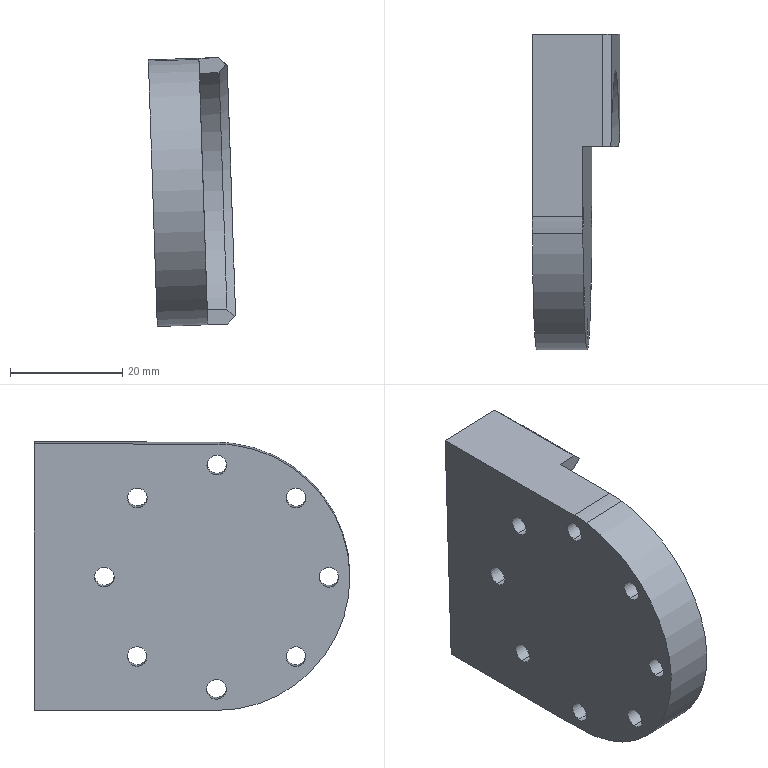Part | STEP file | 2026.6.15-Main Assembly图.sldasm-Part-84 | 1 solid | 42 faces | box 15.538 x 56.282 x 47.929 mm | volume 23654 mm3 | cylinder 27 | plane 14 | cone 1 | commonest cylinder face diameters 3.5 x16 4 x8 47.5 x2 49 x1
STEP:
#1=CARTESIAN_POINT('',(-1524.077,1364.541,3721.229));
#2=VERTEX_POINT('',#1);
#3=CARTESIAN_POINT('',(-1524.077,1364.536,3725.229));
#4=VERTEX_POINT('',#3);
#5=CARTESIAN_POINT('',(-1524.077,1364.538,3723.229));
#6=DIRECTION('',(0.0003632,1.,0.001194));
#7=DIRECTION('',(-0.9994,0.0004028,-0.03334));
#8=AXIS2_PLACEMENT_3D('',#5,#6,#7);
#9=CIRCLE('',#8,2.);
#10=EDGE_CURVE('',#2,#4,#9,.T.);
#11=ORIENTED_EDGE('',*,*,#10,.F.);
#12=CARTESIAN_POINT('',(-1524.075,1372.041,3721.238));
#13=VERTEX_POINT('',#12);
#14=CARTESIAN_POINT('',(-1524.077,1364.541,3721.229));
#15=DIRECTION('',(0.0003632,1.,0.001194));
#16=VECTOR('',#15,1000.);
#17=LINE('',#14,#16);
#18=EDGE_CURVE('',#2,#13,#17,.T.);
#19=ORIENTED_EDGE('',*,*,#18,.T.);
#20=CARTESIAN_POINT('',(-1524.074,1372.036,3725.238));
#21=VERTEX_POINT('',#20);
#22=CARTESIAN_POINT('',(-1524.074,1372.038,3723.238));
#23=DIRECTION('',(-0.0003632,-1.,-0.001194));
#24=DIRECTION('',(-0.9994,0.0004028,-0.03334));
#25=AXIS2_PLACEMENT_3D('',#22,#23,#24);
#26=CIRCLE('',#25,2.);
#27=EDGE_CURVE('',#21,#13,#26,.T.);
#28=ORIENTED_EDGE('',*,*,#27,.F.);
#29=CARTESIAN_POINT('',(-1524.077,1364.536,3725.229));
#30=DIRECTION('',(0.0003632,1.,0.001194));
#31=VECTOR('',#30,1000.);
#32=LINE('',#29,#31);
#33=EDGE_CURVE('',#4,#21,#32,.T.);
#34=ORIENTED_EDGE('',*,*,#33,.F.);
#35=EDGE_LOOP('',(#11,#19,#28,#34));
#36=FACE_OUTER_BOUND('',#35,.T.);
#37=CARTESIAN_POINT('',(-1524.077,1364.538,3723.229));
#38=DIRECTION('',(0.0003632,1.,0.001194));
#39=DIRECTION('',(0.0001943,-0.001194,1.));
#40=AXIS2_PLACEMENT_3D('',#37,#38,#39);
#41=CYLINDRICAL_SURFACE('',#40,2.);
#42=ADVANCED_FACE('',(#36),#41,.F.);
#43=CARTESIAN_POINT('',(-1523.66,1364.551,3712.736));
#44=VERTEX_POINT('',#43);
#45=CARTESIAN_POINT('',(-1523.661,1364.555,3708.736));
#46=VERTEX_POINT('',#45);
#47=CARTESIAN_POINT('',(-1523.66,1364.553,3710.736));
#48=DIRECTION('',(-0.0003632,-1.,-0.001194));
#49=DIRECTION('',(-0.9994,0.0004028,-0.03334));
#50=AXIS2_PLACEMENT_3D('',#47,#48,#49);
#51=CIRCLE('',#50,2.);
#52=EDGE_CURVE('',#44,#46,#51,.T.);
#53=ORIENTED_EDGE('',*,*,#52,.T.);
#54=CARTESIAN_POINT('',(-1523.658,1372.055,3708.745));
#55=VERTEX_POINT('',#54);
#56=CARTESIAN_POINT('',(-1523.661,1364.555,3708.736));
#57=DIRECTION('',(0.0003632,1.,0.001194));
#58=VECTOR('',#57,1000.);
#59=LINE('',#56,#58);
#60=EDGE_CURVE('',#46,#55,#59,.T.);
#61=ORIENTED_EDGE('',*,*,#60,.T.);
#62=CARTESIAN_POINT('',(-1523.657,1372.051,3712.745));
#63=VERTEX_POINT('',#62);
#64=CARTESIAN_POINT('',(-1523.658,1372.053,3710.745));
#65=DIRECTION('',(0.0003632,1.,0.001194));
#66=DIRECTION('',(-0.9994,0.0004028,-0.03334));
#67=AXIS2_PLACEMENT_3D('',#64,#65,#66);
#68=CIRCLE('',#67,2.);
#69=EDGE_CURVE('',#55,#63,#68,.T.);
#70=ORIENTED_EDGE('',*,*,#69,.T.);
#71=CARTESIAN_POINT('',(-1523.66,1364.551,3712.736));
#72=DIRECTION('',(0.0003632,1.,0.001194));
#73=VECTOR('',#72,1000.);
#74=LINE('',#71,#73);
#75=EDGE_CURVE('',#44,#63,#74,.T.);
#76=ORIENTED_EDGE('',*,*,#75,.F.);
#77=EDGE_LOOP('',(#53,#61,#70,#76));
#78=FACE_OUTER_BOUND('',#77,.T.);
#79=CARTESIAN_POINT('',(-1523.66,1364.553,3710.736));
#80=DIRECTION('',(0.0003632,1.,0.001194));
#81=DIRECTION('',(0.0001943,-0.001194,1.));
#82=AXIS2_PLACEMENT_3D('',#79,#80,#81);
#83=CYLINDRICAL_SURFACE('',#82,2.);
#84=ADVANCED_FACE('',(#78),#83,.F.);
#85=CARTESIAN_POINT('',(-1523.243,1364.565,3700.243));
#86=VERTEX_POINT('',#85);
#87=CARTESIAN_POINT('',(-1523.244,1364.57,3696.243));
#88=VERTEX_POINT('',#87);
#89=CARTESIAN_POINT('',(-1523.243,1364.568,3698.243));
#90=DIRECTION('',(-0.0003632,-1.,-0.001194));
#91=DIRECTION('',(-0.9994,0.0004028,-0.03334));
#92=AXIS2_PLACEMENT_3D('',#89,#90,#91);
#93=CIRCLE('',#92,2.);
#94=EDGE_CURVE('',#86,#88,#93,.T.);
#95=ORIENTED_EDGE('',*,*,#94,.T.);
#96=CARTESIAN_POINT('',(-1523.241,1372.07,3696.252));
#97=VERTEX_POINT('',#96);
#98=CARTESIAN_POINT('',(-1523.244,1364.57,3696.243));
#99=DIRECTION('',(0.0003632,1.,0.001194));
#100=VECTOR('',#99,1000.);
#101=LINE('',#98,#100);
#102=EDGE_CURVE('',#88,#97,#101,.T.);
#103=ORIENTED_EDGE('',*,*,#102,.T.);
#104=CARTESIAN_POINT('',(-1523.24,1372.065,3700.252));
#105=VERTEX_POINT('',#104);
#106=CARTESIAN_POINT('',(-1523.241,1372.068,3698.252));
#107=DIRECTION('',(0.0003632,1.,0.001194));
#108=DIRECTION('',(-0.9994,0.0004028,-0.03334));
#109=AXIS2_PLACEMENT_3D('',#106,#107,#108);
#110=CIRCLE('',#109,2.);
#111=EDGE_CURVE('',#97,#105,#110,.T.);
#112=ORIENTED_EDGE('',*,*,#111,.T.);
#113=CARTESIAN_POINT('',(-1523.243,1364.565,3700.243));
#114=DIRECTION('',(0.0003632,1.,0.001194));
#115=VECTOR('',#114,1000.);
#116=LINE('',#113,#115);
#117=EDGE_CURVE('',#86,#105,#116,.T.);
#118=ORIENTED_EDGE('',*,*,#117,.F.);
#119=EDGE_LOOP('',(#95,#103,#112,#118));
#120=FACE_OUTER_BOUND('',#119,.T.);
#121=CARTESIAN_POINT('',(-1523.243,1364.568,3698.243));
#122=DIRECTION('',(0.0003632,1.,0.001194));
#123=DIRECTION('',(0.0001943,-0.001194,1.));
#124=AXIS2_PLACEMENT_3D('',#121,#122,#123);
#125=CYLINDRICAL_SURFACE('',#124,2.);
#126=ADVANCED_FACE('',(#120),#125,.F.);
#127=CARTESIAN_POINT('',(-1522.826,1364.58,3687.75));
#128=VERTEX_POINT('',#127);
#129=CARTESIAN_POINT('',(-1522.827,1364.585,3683.75));
#130=VERTEX_POINT('',#129);
#131=CARTESIAN_POINT('',(-1522.827,1364.583,3685.75));
#132=DIRECTION('',(-0.0003632,-1.,-0.001194));
#133=DIRECTION('',(-0.9994,0.0004028,-0.03334));
#134=AXIS2_PLACEMENT_3D('',#131,#132,#133);
#135=CIRCLE('',#134,2.);
#136=EDGE_CURVE('',#128,#130,#135,.T.);
#137=ORIENTED_EDGE('',*,*,#136,.T.);
#138=CARTESIAN_POINT('',(-1522.824,1372.085,3683.759));
#139=VERTEX_POINT('',#138);
#140=CARTESIAN_POINT('',(-1522.827,1364.585,3683.75));
#141=DIRECTION('',(0.0003632,1.,0.001194));
#142=VECTOR('',#141,1000.);
#143=LINE('',#140,#142);
#144=EDGE_CURVE('',#130,#139,#143,.T.);
#145=ORIENTED_EDGE('',*,*,#144,.T.);
#146=CARTESIAN_POINT('',(-1522.824,1372.08,3687.759));
#147=VERTEX_POINT('',#146);
#148=CARTESIAN_POINT('',(-1522.824,1372.083,3685.759));
#149=DIRECTION('',(0.0003632,1.,0.001194));
#150=DIRECTION('',(-0.9994,0.0004028,-0.03334));
#151=AXIS2_PLACEMENT_3D('',#148,#149,#150);
#152=CIRCLE('',#151,2.);
#153=EDGE_CURVE('',#139,#147,#152,.T.);
#154=ORIENTED_EDGE('',*,*,#153,.T.);
#155=CARTESIAN_POINT('',(-1522.826,1364.58,3687.75));
#156=DIRECTION('',(0.0003632,1.,0.001194));
#157=VECTOR('',#156,1000.);
#158=LINE('',#155,#157);
#159=EDGE_CURVE('',#128,#147,#158,.T.);
#160=ORIENTED_EDGE('',*,*,#159,.F.);
#161=EDGE_LOOP('',(#137,#145,#154,#160));
#162=FACE_OUTER_BOUND('',#161,.T.);
#163=CARTESIAN_POINT('',(-1522.827,1364.583,3685.75));
#164=DIRECTION('',(0.0003632,1.,0.001194));
#165=DIRECTION('',(0.0001943,-0.001194,1.));
#166=AXIS2_PLACEMENT_3D('',#163,#164,#165);
#167=CYLINDRICAL_SURFACE('',#166,2.);
#168=ADVANCED_FACE('',(#162),#167,.F.);
#169=CARTESIAN_POINT('',(-1522.736,1339.811,3682.737));
#170=VERTEX_POINT('',#169);
#171=CARTESIAN_POINT('',(-1522.852,1339.357,3686.205));
#172=VERTEX_POINT('',#171);
#173=CARTESIAN_POINT('',(-1522.794,1339.584,3684.471));
#174=DIRECTION('',(-0.9994,0.0004028,-0.03334));
#175=DIRECTION('',(-0.03311,-0.1296,0.991));
#176=AXIS2_PLACEMENT_3D('',#173,#174,#175);
#177=CIRCLE('',#176,1.75);
#178=EDGE_CURVE('',#170,#172,#177,.T.);
#179=ORIENTED_EDGE('',*,*,#178,.F.);
#180=CARTESIAN_POINT('',(-1531.731,1339.814,3682.436));
#181=VERTEX_POINT('',#180);
#182=CARTESIAN_POINT('',(-1517.739,1339.809,3682.903));
#183=DIRECTION('',(-0.9994,0.0004028,-0.03334));
#184=VECTOR('',#183,1000.);
#185=LINE('',#182,#184);
#186=EDGE_CURVE('',#170,#181,#185,.T.);
#187=ORIENTED_EDGE('',*,*,#186,.T.);
#188=CARTESIAN_POINT('',(-1531.847,1339.361,3685.905));
#189=VERTEX_POINT('',#188);
#190=CARTESIAN_POINT('',(-1531.789,1339.588,3684.171));
#191=DIRECTION('',(0.9994,-0.0004028,0.03334));
#192=DIRECTION('',(-0.03334,-0.001181,0.9994));
#193=AXIS2_PLACEMENT_3D('',#190,#191,#192);
#194=CIRCLE('',#193,1.75);
#195=EDGE_CURVE('',#189,#181,#194,.T.);
#196=ORIENTED_EDGE('',*,*,#195,.F.);
#197=CARTESIAN_POINT('',(-1517.855,1339.355,3686.372));
#198=DIRECTION('',(-0.9994,0.0004028,-0.03334));
#199=VECTOR('',#198,1000.);
#200=LINE('',#197,#199);
#201=EDGE_CURVE('',#172,#189,#200,.T.);
#202=ORIENTED_EDGE('',*,*,#201,.F.);
#203=EDGE_LOOP('',(#179,#187,#196,#202));
#204=FACE_OUTER_BOUND('',#203,.T.);
#205=CARTESIAN_POINT('',(-1517.797,1339.582,3684.637));
#206=DIRECTION('',(-0.9994,0.0004028,-0.03334));
#207=DIRECTION('',(-0.03311,-0.1296,0.991));
#208=AXIS2_PLACEMENT_3D('',#205,#206,#207);
#209=CYLINDRICAL_SURFACE('',#208,1.75);
#210=ADVANCED_FACE('',(#204),#209,.F.);
#211=CARTESIAN_POINT('',(-1524.07,1339.764,3722.714));
#212=VERTEX_POINT('',#211);
#213=CARTESIAN_POINT('',(-1524.186,1339.31,3726.183));
#214=VERTEX_POINT('',#213);
#215=CARTESIAN_POINT('',(-1524.128,1339.537,3724.449));
#216=DIRECTION('',(-0.9994,0.0004028,-0.03334));
#217=DIRECTION('',(-0.03311,-0.1296,0.991));
#218=AXIS2_PLACEMENT_3D('',#215,#216,#217);
#219=CIRCLE('',#218,1.75);
#220=EDGE_CURVE('',#212,#214,#219,.T.);
#221=ORIENTED_EDGE('',*,*,#220,.F.);
#222=CARTESIAN_POINT('',(-1533.065,1339.767,3722.414));
#223=VERTEX_POINT('',#222);
#224=CARTESIAN_POINT('',(-1519.073,1339.762,3722.881));
#225=DIRECTION('',(-0.9994,0.0004028,-0.03334));
#226=VECTOR('',#225,1000.);
#227=LINE('',#224,#226);
#228=EDGE_CURVE('',#212,#223,#227,.T.);
#229=ORIENTED_EDGE('',*,*,#228,.T.);
#230=CARTESIAN_POINT('',(-1533.181,1339.314,3725.883));
#231=VERTEX_POINT('',#230);
#232=CARTESIAN_POINT('',(-1533.123,1339.54,3724.148));
#233=DIRECTION('',(0.9994,-0.0004028,0.03334));
#234=DIRECTION('',(-0.03334,-0.001181,0.9994));
#235=AXIS2_PLACEMENT_3D('',#232,#233,#234);
#236=CIRCLE('',#235,1.75);
#237=EDGE_CURVE('',#231,#223,#236,.T.);
#238=ORIENTED_EDGE('',*,*,#237,.F.);
#239=CARTESIAN_POINT('',(-1519.188,1339.308,3726.349));
#240=DIRECTION('',(-0.9994,0.0004028,-0.03334));
#241=VECTOR('',#240,1000.);
#242=LINE('',#239,#241);
#243=EDGE_CURVE('',#214,#231,#242,.T.);
#244=ORIENTED_EDGE('',*,*,#243,.F.);
#245=EDGE_LOOP('',(#221,#229,#238,#244));
#246=FACE_OUTER_BOUND('',#245,.T.);
#247=CARTESIAN_POINT('',(-1519.131,1339.535,3724.615));
#248=DIRECTION('',(-0.9994,0.0004028,-0.03334));
#249=DIRECTION('',(-0.03311,-0.1296,0.991));
#250=AXIS2_PLACEMENT_3D('',#247,#248,#249);
#251=CYLINDRICAL_SURFACE('',#250,1.75);
#252=ADVANCED_FACE('',(#246),#251,.F.);
#253=CARTESIAN_POINT('',(-1523.88,1325.628,3716.843));
#254=VERTEX_POINT('',#253);
#255=CARTESIAN_POINT('',(-1523.996,1325.175,3720.311));
#256=VERTEX_POINT('',#255);
#257=CARTESIAN_POINT('',(-1523.938,1325.402,3718.577));
#258=DIRECTION('',(-0.9994,0.0004028,-0.03334));
#259=DIRECTION('',(-0.03311,-0.1296,0.991));
#260=AXIS2_PLACEMENT_3D('',#257,#258,#259);
#261=CIRCLE('',#260,1.75);
#262=EDGE_CURVE('',#254,#256,#261,.T.);
#263=ORIENTED_EDGE('',*,*,#262,.F.);
#264=CARTESIAN_POINT('',(-1532.875,1325.632,3716.543));
#265=VERTEX_POINT('',#264);
#266=CARTESIAN_POINT('',(-1518.882,1325.626,3717.009));
#267=DIRECTION('',(-0.9994,0.0004028,-0.03334));
#268=VECTOR('',#267,1000.);
#269=LINE('',#266,#268);
#270=EDGE_CURVE('',#254,#265,#269,.T.);
#271=ORIENTED_EDGE('',*,*,#270,.T.);
#272=CARTESIAN_POINT('',(-1532.991,1325.178,3720.011));
#273=VERTEX_POINT('',#272);
#274=CARTESIAN_POINT('',(-1532.933,1325.405,3718.277));
#275=DIRECTION('',(0.9994,-0.0004028,0.03334));
#276=DIRECTION('',(-0.03334,-0.001181,0.9994));
#277=AXIS2_PLACEMENT_3D('',#274,#275,#276);
#278=CIRCLE('',#277,1.75);
#279=EDGE_CURVE('',#273,#265,#278,.T.);
#280=ORIENTED_EDGE('',*,*,#279,.F.);
#281=CARTESIAN_POINT('',(-1518.998,1325.173,3720.478));
#282=DIRECTION('',(-0.9994,0.0004028,-0.03334));
#283=VECTOR('',#282,1000.);
#284=LINE('',#281,#283);
#285=EDGE_CURVE('',#256,#273,#284,.T.);
#286=ORIENTED_EDGE('',*,*,#285,.F.);
#287=EDGE_LOOP('',(#263,#271,#280,#286));
#288=FACE_OUTER_BOUND('',#287,.T.);
#289=CARTESIAN_POINT('',(-1518.94,1325.4,3718.744));
#290=DIRECTION('',(-0.9994,0.0004028,-0.03334));
#291=DIRECTION('',(-0.03311,-0.1296,0.991));
#292=AXIS2_PLACEMENT_3D('',#289,#290,#291);
#293=CYLINDRICAL_SURFACE('',#292,1.75);
#294=ADVANCED_FACE('',(#288),#293,.F.);
#295=CARTESIAN_POINT('',(-1523.869,1353.913,3716.877));
#296=VERTEX_POINT('',#295);
#297=CARTESIAN_POINT('',(-1523.985,1353.459,3720.345));
#298=VERTEX_POINT('',#297);
#299=CARTESIAN_POINT('',(-1523.927,1353.686,3718.611));
#300=DIRECTION('',(-0.9994,0.0004028,-0.03334));
#301=DIRECTION('',(-0.03311,-0.1296,0.991));
#302=AXIS2_PLACEMENT_3D('',#299,#300,#301);
#303=CIRCLE('',#302,1.75);
#304=EDGE_CURVE('',#296,#298,#303,.T.);
#305=ORIENTED_EDGE('',*,*,#304,.F.);
#306=CARTESIAN_POINT('',(-1532.864,1353.916,3716.576));
#307=VERTEX_POINT('',#306);
#308=CARTESIAN_POINT('',(-1518.872,1353.911,3717.043));
#309=DIRECTION('',(-0.9994,0.0004028,-0.03334));
#310=VECTOR('',#309,1000.);
#311=LINE('',#308,#310);
#312=EDGE_CURVE('',#296,#307,#311,.T.);
#313=ORIENTED_EDGE('',*,*,#312,.T.);
#314=CARTESIAN_POINT('',(-1532.98,1353.463,3720.045));
#315=VERTEX_POINT('',#314);
#316=CARTESIAN_POINT('',(-1532.922,1353.69,3718.311));
#317=DIRECTION('',(0.9994,-0.0004028,0.03334));
#318=DIRECTION('',(-0.03334,-0.001181,0.9994));
#319=AXIS2_PLACEMENT_3D('',#316,#317,#318);
#320=CIRCLE('',#319,1.75);
#321=EDGE_CURVE('',#315,#307,#320,.T.);
#322=ORIENTED_EDGE('',*,*,#321,.F.);
#323=CARTESIAN_POINT('',(-1518.988,1353.457,3720.512));
#324=DIRECTION('',(-0.9994,0.0004028,-0.03334));
#325=VECTOR('',#324,1000.);
#326=LINE('',#323,#325);
#327=EDGE_CURVE('',#298,#315,#326,.T.);
#328=ORIENTED_EDGE('',*,*,#327,.F.);
#329=EDGE_LOOP('',(#305,#313,#322,#328));
#330=FACE_OUTER_BOUND('',#329,.T.);
#331=CARTESIAN_POINT('',(-1518.93,1353.684,3718.777));
#332=DIRECTION('',(-0.9994,0.0004028,-0.03334));
#333=DIRECTION('',(-0.03311,-0.1296,0.991));
#334=AXIS2_PLACEMENT_3D('',#331,#332,#333);
#335=CYLINDRICAL_SURFACE('',#334,1.75);
#336=ADVANCED_FACE('',(#330),#335,.F.);
#337=CARTESIAN_POINT('',(-1523.41,1319.787,3702.702));
#338=VERTEX_POINT('',#337);
#339=CARTESIAN_POINT('',(-1523.526,1319.334,3706.17));
#340=VERTEX_POINT('',#339);
#341=CARTESIAN_POINT('',(-1523.468,1319.56,3704.436));
#342=DIRECTION('',(-0.9994,0.0004028,-0.03334));
#343=DIRECTION('',(-0.03311,-0.1296,0.991));
#344=AXIS2_PLACEMENT_3D('',#341,#342,#343);
#345=CIRCLE('',#344,1.75);
#346=EDGE_CURVE('',#338,#340,#345,.T.);
#347=ORIENTED_EDGE('',*,*,#346,.F.);
#348=CARTESIAN_POINT('',(-1532.405,1319.791,3702.401));
#349=VERTEX_POINT('',#348);
#350=CARTESIAN_POINT('',(-1518.413,1319.785,3702.868));
#351=DIRECTION('',(-0.9994,0.0004028,-0.03334));
#352=VECTOR('',#351,1000.);
#353=LINE('',#350,#352);
#354=EDGE_CURVE('',#338,#349,#353,.T.);
#355=ORIENTED_EDGE('',*,*,#354,.T.);
#356=CARTESIAN_POINT('',(-1532.521,1319.337,3705.87));
#357=VERTEX_POINT('',#356);
#358=CARTESIAN_POINT('',(-1532.463,1319.564,3704.136));
#359=DIRECTION('',(0.9994,-0.0004028,0.03334));
#360=DIRECTION('',(-0.03334,-0.001181,0.9994));
#361=AXIS2_PLACEMENT_3D('',#358,#359,#360);
#362=CIRCLE('',#361,1.75);
#363=EDGE_CURVE('',#357,#349,#362,.T.);
#364=ORIENTED_EDGE('',*,*,#363,.F.);
#365=CARTESIAN_POINT('',(-1518.529,1319.332,3706.337));
#366=DIRECTION('',(-0.9994,0.0004028,-0.03334));
#367=VECTOR('',#366,1000.);
#368=LINE('',#365,#367);
#369=EDGE_CURVE('',#340,#357,#368,.T.);
#370=ORIENTED_EDGE('',*,*,#369,.F.);
#371=EDGE_LOOP('',(#347,#355,#364,#370));
#372=FACE_OUTER_BOUND('',#371,.T.);
#373=CARTESIAN_POINT('',(-1518.471,1319.558,3704.602));
#374=DIRECTION('',(-0.9994,0.0004028,-0.03334));
#375=DIRECTION('',(-0.03311,-0.1296,0.991));
#376=AXIS2_PLACEMENT_3D('',#373,#374,#375);
#377=CYLINDRICAL_SURFACE('',#376,1.75);
#378=ADVANCED_FACE('',(#372),#377,.F.);
#379=CARTESIAN_POINT('',(-1523.396,1359.787,3702.749));
#380=VERTEX_POINT('',#379);
#381=CARTESIAN_POINT('',(-1523.512,1359.334,3706.218));
#382=VERTEX_POINT('',#381);
#383=CARTESIAN_POINT('',(-1523.454,1359.56,3704.484));
#384=DIRECTION('',(-0.9994,0.0004028,-0.03334));
#385=DIRECTION('',(-0.03311,-0.1296,0.991));
#386=AXIS2_PLACEMENT_3D('',#383,#384,#385);
#387=CIRCLE('',#386,1.75);
#388=EDGE_CURVE('',#380,#382,#387,.T.);
#389=ORIENTED_EDGE('',*,*,#388,.F.);
#390=CARTESIAN_POINT('',(-1532.391,1359.791,3702.449));
#391=VERTEX_POINT('',#390);
#392=CARTESIAN_POINT('',(-1518.399,1359.785,3702.916));
#393=DIRECTION('',(-0.9994,0.0004028,-0.03334));
#394=VECTOR('',#393,1000.);
#395=LINE('',#392,#394);
#396=EDGE_CURVE('',#380,#391,#395,.T.);
#397=ORIENTED_EDGE('',*,*,#396,.T.);
#398=CARTESIAN_POINT('',(-1532.507,1359.337,3705.918));
#399=VERTEX_POINT('',#398);
#400=CARTESIAN_POINT('',(-1532.449,1359.564,3704.183));
#401=DIRECTION('',(0.9994,-0.0004028,0.03334));
#402=DIRECTION('',(-0.03334,-0.001181,0.9994));
#403=AXIS2_PLACEMENT_3D('',#400,#401,#402);
#404=CIRCLE('',#403,1.75);
#405=EDGE_CURVE('',#399,#391,#404,.T.);
#406=ORIENTED_EDGE('',*,*,#405,.F.);
#407=CARTESIAN_POINT('',(-1518.514,1359.332,3706.385));
#408=DIRECTION('',(-0.9994,0.0004028,-0.03334));
#409=VECTOR('',#408,1000.);
#410=LINE('',#407,#409);
#411=EDGE_CURVE('',#382,#399,#410,.T.);
#412=ORIENTED_EDGE('',*,*,#411,.F.);
#413=EDGE_LOOP('',(#389,#397,#406,#412));
#414=FACE_OUTER_BOUND('',#413,.T.);
#415=CARTESIAN_POINT('',(-1518.456,1359.558,3704.65));
#416=DIRECTION('',(-0.9994,0.0004028,-0.03334));
#417=DIRECTION('',(-0.03311,-0.1296,0.991));
#418=AXIS2_PLACEMENT_3D('',#415,#416,#417);
#419=CYLINDRICAL_SURFACE('',#418,1.75);
#420=ADVANCED_FACE('',(#414),#419,.F.);
#421=CARTESIAN_POINT('',(-1522.937,1325.662,3688.574));
#422=VERTEX_POINT('',#421);
#423=CARTESIAN_POINT('',(-1523.053,1325.208,3692.043));
#424=VERTEX_POINT('',#423);
#425=CARTESIAN_POINT('',(-1522.995,1325.435,3690.309));
#426=DIRECTION('',(-0.9994,0.0004028,-0.03334));
#427=DIRECTION('',(-0.03311,-0.1296,0.991));
#428=AXIS2_PLACEMENT_3D('',#425,#426,#427);
#429=CIRCLE('',#428,1.75);
#430=EDGE_CURVE('',#422,#424,#429,.T.);
#431=ORIENTED_EDGE('',*,*,#430,.F.);
#432=CARTESIAN_POINT('',(-1531.932,1325.665,3688.274));
#433=VERTEX_POINT('',#432);
#434=CARTESIAN_POINT('',(-1517.939,1325.66,3688.741));
#435=DIRECTION('',(-0.9994,0.0004028,-0.03334));
#436=VECTOR('',#435,1000.);
#437=LINE('',#434,#436);
#438=EDGE_CURVE('',#422,#433,#437,.T.);
#439=ORIENTED_EDGE('',*,*,#438,.T.);
#440=CARTESIAN_POINT('',(-1532.048,1325.212,3691.743));
#441=VERTEX_POINT('',#440);
#442=CARTESIAN_POINT('',(-1531.99,1325.439,3690.008));
#443=DIRECTION('',(0.9994,-0.0004028,0.03334));
#444=DIRECTION('',(-0.03334,-0.001181,0.9994));
#445=AXIS2_PLACEMENT_3D('',#442,#443,#444);
#446=CIRCLE('',#445,1.75);
#447=EDGE_CURVE('',#441,#433,#446,.T.);
#448=ORIENTED_EDGE('',*,*,#447,.F.);
#449=CARTESIAN_POINT('',(-1518.055,1325.206,3692.209));
#450=DIRECTION('',(-0.9994,0.0004028,-0.03334));
#451=VECTOR('',#450,1000.);
#452=LINE('',#449,#451);
#453=EDGE_CURVE('',#424,#441,#452,.T.);
#454=ORIENTED_EDGE('',*,*,#453,.F.);
#455=EDGE_LOOP('',(#431,#439,#448,#454));
#456=FACE_OUTER_BOUND('',#455,.T.);
#457=CARTESIAN_POINT('',(-1517.997,1325.433,3690.475));
#458=DIRECTION('',(-0.9994,0.0004028,-0.03334));
#459=DIRECTION('',(-0.03311,-0.1296,0.991));
#460=AXIS2_PLACEMENT_3D('',#457,#458,#459);
#461=CYLINDRICAL_SURFACE('',#460,1.75);
#462=ADVANCED_FACE('',(#456),#461,.F.);
#463=CARTESIAN_POINT('',(-1522.926,1353.946,3688.608));
#464=VERTEX_POINT('',#463);
#465=CARTESIAN_POINT('',(-1523.042,1353.493,3692.077));
#466=VERTEX_POINT('',#465);
#467=CARTESIAN_POINT('',(-1522.984,1353.719,3690.342));
#468=DIRECTION('',(-0.9994,0.0004028,-0.03334));
#469=DIRECTION('',(-0.03311,-0.1296,0.991));
#470=AXIS2_PLACEMENT_3D('',#467,#468,#469);
#471=CIRCLE('',#470,1.75);
#472=EDGE_CURVE('',#464,#466,#471,.T.);
#473=ORIENTED_EDGE('',*,*,#472,.F.);
#474=CARTESIAN_POINT('',(-1531.921,1353.95,3688.308));
#475=VERTEX_POINT('',#474);
#476=CARTESIAN_POINT('',(-1517.929,1353.944,3688.775));
#477=DIRECTION('',(-0.9994,0.0004028,-0.03334));
#478=VECTOR('',#477,1000.);
#479=LINE('',#476,#478);
#480=EDGE_CURVE('',#464,#475,#479,.T.);
#481=ORIENTED_EDGE('',*,*,#480,.T.);
#482=CARTESIAN_POINT('',(-1532.037,1353.496,3691.776));
#483=VERTEX_POINT('',#482);
#484=CARTESIAN_POINT('',(-1531.979,1353.723,3690.042));
#485=DIRECTION('',(0.9994,-0.0004028,0.03334));
#486=DIRECTION('',(-0.03334,-0.001181,0.9994));
#487=AXIS2_PLACEMENT_3D('',#484,#485,#486);
#488=CIRCLE('',#487,1.75);
#489=EDGE_CURVE('',#483,#475,#488,.T.);
#490=ORIENTED_EDGE('',*,*,#489,.F.);
#491=CARTESIAN_POINT('',(-1518.045,1353.49,3692.243));
#492=DIRECTION('',(-0.9994,0.0004028,-0.03334));
#493=VECTOR('',#492,1000.);
#494=LINE('',#491,#493);
#495=EDGE_CURVE('',#466,#483,#494,.T.);
#496=ORIENTED_EDGE('',*,*,#495,.F.);
#497=EDGE_LOOP('',(#473,#481,#490,#496));
#498=FACE_OUTER_BOUND('',#497,.T.);
#499=CARTESIAN_POINT('',(-1517.987,1353.717,3690.509));
#500=DIRECTION('',(-0.9994,0.0004028,-0.03334));
#501=DIRECTION('',(-0.03311,-0.1296,0.991));
#502=AXIS2_PLACEMENT_3D('',#499,#500,#501);
#503=CYLINDRICAL_SURFACE('',#502,1.75);
#504=ADVANCED_FACE('',(#498),#503,.F.);
#505=CARTESIAN_POINT('',(-1522.669,1339.589,3680.723));
#506=VERTEX_POINT('',#505);
#507=CARTESIAN_POINT('',(-1524.247,1336.483,3727.996));
#508=VERTEX_POINT('',#507);
#509=CARTESIAN_POINT('',(-1523.461,1339.56,3704.46));
#510=DIRECTION('',(-0.9994,0.0004028,-0.03334));
#511=DIRECTION('',(-0.03334,-0.001181,0.9994));
#512=AXIS2_PLACEMENT_3D('',#509,#510,#511);
#513=CIRCLE('',#512,23.75);
#514=EDGE_CURVE('',#506,#508,#513,.T.);
#515=ORIENTED_EDGE('',*,*,#514,.T.);
#516=CARTESIAN_POINT('',(-1533.242,1336.486,3727.696));
#517=VERTEX_POINT('',#516);
#518=CARTESIAN_POINT('',(-1519.25,1336.481,3728.163));
#519=DIRECTION('',(-0.9994,0.0004028,-0.03334));
#520=VECTOR('',#519,1000.);
#521=LINE('',#518,#520);
#522=EDGE_CURVE('',#508,#517,#521,.T.);
#523=ORIENTED_EDGE('',*,*,#522,.T.);
#524=CARTESIAN_POINT('',(-1531.664,1339.592,3680.423));
#525=VERTEX_POINT('',#524);
#526=CARTESIAN_POINT('',(-1532.456,1339.564,3704.16));
#527=DIRECTION('',(-0.9994,0.0004028,-0.03334));
#528=DIRECTION('',(-0.03334,-0.001181,0.9994));
#529=AXIS2_PLACEMENT_3D('',#526,#527,#528);
#530=CIRCLE('',#529,23.75);
#531=EDGE_CURVE('',#525,#517,#530,.T.);
#532=ORIENTED_EDGE('',*,*,#531,.F.);
#533=CARTESIAN_POINT('',(-1517.672,1339.586,3680.89));
#534=DIRECTION('',(-0.9994,0.0004028,-0.03334));
#535=VECTOR('',#534,1000.);
#536=LINE('',#533,#535);
#537=EDGE_CURVE('',#506,#525,#536,.T.);
#538=ORIENTED_EDGE('',*,*,#537,.F.);
#539=EDGE_LOOP('',(#515,#523,#532,#538));
#540=FACE_OUTER_BOUND('',#539,.T.);
#541=CARTESIAN_POINT('',(-1518.464,1339.558,3704.626));
#542=DIRECTION('',(-0.9994,0.0004028,-0.03334));
#543=DIRECTION('',(-0.03311,-0.1296,0.991));
#544=AXIS2_PLACEMENT_3D('',#541,#542,#543);
#545=CYLINDRICAL_SURFACE('',#544,23.75);
#546=ADVANCED_FACE('',(#540),#545,.T.);
#547=CARTESIAN_POINT('',(-1519.159,1372.087,3680.878));
#548=VERTEX_POINT('',#547);
#549=CARTESIAN_POINT('',(-1531.652,1372.092,3680.462));
#550=VERTEX_POINT('',#549);
#551=CARTESIAN_POINT('',(-1517.66,1372.086,3680.928));
#552=DIRECTION('',(-0.9994,0.0004028,-0.03334));
#553=VECTOR('',#552,1000.);
#554=LINE('',#551,#553);
#555=EDGE_CURVE('',#548,#550,#554,.T.);
#556=ORIENTED_EDGE('',*,*,#555,.F.);
#557=CARTESIAN_POINT('',(-1519.167,1352.087,3680.854));
#558=VERTEX_POINT('',#557);
#559=CARTESIAN_POINT('',(-1519.167,1352.087,3680.854));
#560=DIRECTION('',(-0.0003632,-1.,-0.001194));
#561=VECTOR('',#560,1000.);
#562=LINE('',#559,#561);
#563=EDGE_CURVE('',#548,#558,#562,.T.);
#564=ORIENTED_EDGE('',*,*,#563,.T.);
#565=CARTESIAN_POINT('',(-1522.665,1352.088,3680.738));
#566=VERTEX_POINT('',#565);
#567=CARTESIAN_POINT('',(-1517.667,1352.086,3680.904));
#568=DIRECTION('',(-0.9994,0.0004028,-0.03334));
#569=VECTOR('',#568,1000.);
#570=LINE('',#567,#569);
#571=EDGE_CURVE('',#558,#566,#570,.T.);
#572=ORIENTED_EDGE('',*,*,#571,.T.);
#573=CARTESIAN_POINT('',(-1522.665,1352.088,3680.738));
#574=DIRECTION('',(-0.0003632,-1.,-0.001194));
#575=VECTOR('',#574,1000.);
#576=LINE('',#573,#575);
#577=EDGE_CURVE('',#566,#506,#576,.T.);
#578=ORIENTED_EDGE('',*,*,#577,.T.);
#579=ORIENTED_EDGE('',*,*,#537,.T.);
#580=CARTESIAN_POINT('',(-1531.652,1372.092,3680.462));
#581=DIRECTION('',(-0.0003632,-1.,-0.001194));
#582=VECTOR('',#581,1000.);
#583=LINE('',#580,#582);
#584=EDGE_CURVE('',#550,#525,#583,.T.);
#585=ORIENTED_EDGE('',*,*,#584,.F.);
#586=EDGE_LOOP('',(#556,#564,#572,#578,#579,#585));
#587=FACE_OUTER_BOUND('',#586,.T.);
#588=CARTESIAN_POINT('',(-1517.66,1372.086,3680.928));
#589=DIRECTION('',(0.03334,0.001181,-0.9994));
#590=DIRECTION('',(-0.003979,1.,0.001049));
#591=AXIS2_PLACEMENT_3D('',#588,#589,#590);
#592=PLANE('',#591);
#593=ADVANCED_FACE('',(#587),#592,.T.);
#594=CARTESIAN_POINT('',(-1520.75,1352.031,3728.328));
#595=VERTEX_POINT('',#594);
#596=CARTESIAN_POINT('',(-1524.248,1352.032,3728.211));
#597=VERTEX_POINT('',#596);
#598=CARTESIAN_POINT('',(-1519.251,1352.03,3728.378));
#599=DIRECTION('',(-0.9994,0.0004028,-0.03334));
#600=VECTOR('',#599,1000.);
#601=LINE('',#598,#600);
#602=EDGE_CURVE('',#595,#597,#601,.T.);
#603=ORIENTED_EDGE('',*,*,#602,.F.);
#604=CARTESIAN_POINT('',(-1520.743,1372.031,3728.352));
#605=VERTEX_POINT('',#604);
#606=CARTESIAN_POINT('',(-1520.743,1372.031,3728.352));
#607=DIRECTION('',(0.0003632,1.,0.001194));
#608=VECTOR('',#607,1000.);
#609=LINE('',#606,#608);
#610=EDGE_CURVE('',#595,#605,#609,.T.);
#611=ORIENTED_EDGE('',*,*,#610,.T.);
#612=CARTESIAN_POINT('',(-1533.236,1372.036,3727.935));
#613=VERTEX_POINT('',#612);
#614=CARTESIAN_POINT('',(-1519.244,1372.03,3728.402));
#615=DIRECTION('',(-0.9994,0.0004028,-0.03334));
#616=VECTOR('',#615,1000.);
#617=LINE('',#614,#616);
#618=EDGE_CURVE('',#605,#613,#617,.T.);
#619=ORIENTED_EDGE('',*,*,#618,.T.);
#620=CARTESIAN_POINT('',(-1533.248,1339.536,3727.896));
#621=VERTEX_POINT('',#620);
#622=CARTESIAN_POINT('',(-1533.248,1339.536,3727.896));
#623=DIRECTION('',(0.0003632,1.,0.001194));
#624=VECTOR('',#623,1000.);
#625=LINE('',#622,#624);
#626=EDGE_CURVE('',#621,#613,#625,.T.);
#627=ORIENTED_EDGE('',*,*,#626,.F.);
#628=CARTESIAN_POINT('',(-1524.253,1339.532,3728.196));
#629=VERTEX_POINT('',#628);
#630=CARTESIAN_POINT('',(-1519.256,1339.53,3728.363));
#631=DIRECTION('',(-0.9994,0.0004028,-0.03334));
#632=VECTOR('',#631,1000.);
#633=LINE('',#630,#632);
#634=EDGE_CURVE('',#629,#621,#633,.T.);
#635=ORIENTED_EDGE('',*,*,#634,.F.);
#636=CARTESIAN_POINT('',(-1524.253,1339.532,3728.196));
#637=DIRECTION('',(0.0003632,1.,0.001194));
#638=VECTOR('',#637,1000.);
#639=LINE('',#636,#638);
#640=EDGE_CURVE('',#629,#597,#639,.T.);
#641=ORIENTED_EDGE('',*,*,#640,.T.);
#642=EDGE_LOOP('',(#603,#611,#619,#627,#635,#641));
#643=FACE_OUTER_BOUND('',#642,.T.);
#644=CARTESIAN_POINT('',(-1519.256,1339.53,3728.363));
#645=DIRECTION('',(-0.03334,-0.001181,0.9994));
#646=DIRECTION('',(0.003979,-1.,-0.001049));
#647=AXIS2_PLACEMENT_3D('',#644,#645,#646);
#648=PLANE('',#647);
#649=ADVANCED_FACE('',(#643),#648,.T.);
#650=ORIENTED_EDGE('',*,*,#522,.F.);
#651=CARTESIAN_POINT('',(-1523.461,1339.56,3704.46));
#652=DIRECTION('',(-0.9994,0.0004028,-0.03334));
#653=DIRECTION('',(-0.03334,-0.001181,0.9994));
#654=AXIS2_PLACEMENT_3D('',#651,#652,#653);
#655=CIRCLE('',#654,23.75);
#656=EDGE_CURVE('',#508,#629,#655,.T.);
#657=ORIENTED_EDGE('',*,*,#656,.T.);
#658=ORIENTED_EDGE('',*,*,#634,.T.);
#659=CARTESIAN_POINT('',(-1532.456,1339.564,3704.16));
#660=DIRECTION('',(-0.9994,0.0004028,-0.03334));
#661=DIRECTION('',(-0.03334,-0.001181,0.9994));
#662=AXIS2_PLACEMENT_3D('',#659,#660,#661);
#663=CIRCLE('',#662,23.75);
#664=EDGE_CURVE('',#517,#621,#663,.T.);
#665=ORIENTED_EDGE('',*,*,#664,.F.);
#666=EDGE_LOOP('',(#650,#657,#658,#665));
#667=FACE_OUTER_BOUND('',#666,.T.);
#668=CARTESIAN_POINT('',(-1518.464,1339.558,3704.626));
#669=DIRECTION('',(-0.9994,0.0004028,-0.03334));
#670=DIRECTION('',(-0.03311,-0.1296,0.991));
#671=AXIS2_PLACEMENT_3D('',#668,#669,#670);
#672=CYLINDRICAL_SURFACE('',#671,23.75);
#673=ADVANCED_FACE('',(#667),#672,.T.);
#674=ORIENTED_EDGE('',*,*,#27,.T.);
#675=CARTESIAN_POINT('',(-1524.074,1372.038,3723.238));
#676=DIRECTION('',(-0.0003632,-1.,-0.001194));
#677=DIRECTION('',(-0.9994,0.0004028,-0.03334));
#678=AXIS2_PLACEMENT_3D('',#675,#676,#677);
#679=CIRCLE('',#678,2.);
#680=EDGE_CURVE('',#13,#21,#679,.T.);
#681=ORIENTED_EDGE('',*,*,#680,.T.);
#682=EDGE_LOOP('',(#674,#681));
#683=FACE_BOUND('',#682,.T.);
#684=CARTESIAN_POINT('',(-1523.658,1372.053,3710.745));
#685=DIRECTION('',(0.0003632,1.,0.001194));
#686=DIRECTION('',(-0.9994,0.0004028,-0.03334));
#687=AXIS2_PLACEMENT_3D('',#684,#685,#686);
#688=CIRCLE('',#687,2.);
#689=EDGE_CURVE('',#63,#55,#688,.T.);
#690=ORIENTED_EDGE('',*,*,#689,.F.);
#691=ORIENTED_EDGE('',*,*,#69,.F.);
#692=EDGE_LOOP('',(#690,#691));
#693=FACE_BOUND('',#692,.T.);
#694=CARTESIAN_POINT('',(-1523.241,1372.068,3698.252));
#695=DIRECTION('',(0.0003632,1.,0.001194));
#696=DIRECTION('',(-0.9994,0.0004028,-0.03334));
#697=AXIS2_PLACEMENT_3D('',#694,#695,#696);
#698=CIRCLE('',#697,2.);
#699=EDGE_CURVE('',#105,#97,#698,.T.);
#700=ORIENTED_EDGE('',*,*,#699,.F.);
#701=ORIENTED_EDGE('',*,*,#111,.F.);
#702=EDGE_LOOP('',(#700,#701));
#703=FACE_BOUND('',#702,.T.);
#704=CARTESIAN_POINT('',(-1522.824,1372.083,3685.759));
#705=DIRECTION('',(0.0003632,1.,0.001194));
#706=DIRECTION('',(-0.9994,0.0004028,-0.03334));
#707=AXIS2_PLACEMENT_3D('',#704,#705,#706);
#708=CIRCLE('',#707,2.);
#709=EDGE_CURVE('',#147,#139,#708,.T.);
#710=ORIENTED_EDGE('',*,*,#709,.F.);
#711=ORIENTED_EDGE('',*,*,#153,.F.);
#712=EDGE_LOOP('',(#710,#711));
#713=FACE_BOUND('',#712,.T.);
#714=CARTESIAN_POINT('',(-1519.194,1372.032,3726.903));
#715=VERTEX_POINT('',#714);
#716=CARTESIAN_POINT('',(-1517.71,1372.085,3682.428));
#717=VERTEX_POINT('',#716);
#718=CARTESIAN_POINT('',(-1519.244,1372.03,3728.402));
#719=DIRECTION('',(0.03334,0.001181,-0.9994));
#720=VECTOR('',#719,1000.);
#721=LINE('',#718,#720);
#722=EDGE_CURVE('',#715,#717,#721,.T.);
#723=ORIENTED_EDGE('',*,*,#722,.T.);
#724=CARTESIAN_POINT('',(-1495.49,1372.048,3706.182));
#725=DIRECTION('',(-0.6831,0.00112,-0.7303));
#726=VECTOR('',#725,1000.);
#727=LINE('',#724,#726);
#728=EDGE_CURVE('',#717,#548,#727,.T.);
#729=ORIENTED_EDGE('',*,*,#728,.T.);
#730=ORIENTED_EDGE('',*,*,#555,.T.);
#731=CARTESIAN_POINT('',(-1533.236,1372.036,3727.935));
#732=DIRECTION('',(0.03334,0.001181,-0.9994));
#733=VECTOR('',#732,1000.);
#734=LINE('',#731,#733);
#735=EDGE_CURVE('',#613,#550,#734,.T.);
#736=ORIENTED_EDGE('',*,*,#735,.F.);
#737=ORIENTED_EDGE('',*,*,#618,.F.);
#738=CARTESIAN_POINT('',(-1519.968,1372.032,3727.627));
#739=DIRECTION('',(0.7303,0.0005501,-0.6831));
#740=VECTOR('',#739,1000.);
#741=LINE('',#738,#740);
#742=EDGE_CURVE('',#605,#715,#741,.T.);
#743=ORIENTED_EDGE('',*,*,#742,.T.);
#744=EDGE_LOOP('',(#723,#729,#730,#736,#737,#743));
#745=FACE_OUTER_BOUND('',#744,.T.);
#746=CARTESIAN_POINT('',(-1519.244,1372.03,3728.402));
#747=DIRECTION('',(0.0003632,1.,0.001194));
#748=DIRECTION('',(0.0001943,-0.001194,1.));
#749=AXIS2_PLACEMENT_3D('',#746,#747,#748);
#750=PLANE('',#749);
#751=ADVANCED_FACE('',(#683,#693,#703,#713,#745),#750,.T.);
#752=ORIENTED_EDGE('',*,*,#480,.F.);
#753=CARTESIAN_POINT('',(-1522.984,1353.719,3690.342));
#754=DIRECTION('',(-0.9994,0.0004028,-0.03334));
#755=DIRECTION('',(-0.03311,-0.1296,0.991));
#756=AXIS2_PLACEMENT_3D('',#753,#754,#755);
#757=CIRCLE('',#756,1.75);
#758=EDGE_CURVE('',#466,#464,#757,.T.);
#759=ORIENTED_EDGE('',*,*,#758,.F.);
#760=ORIENTED_EDGE('',*,*,#495,.T.);
#761=CARTESIAN_POINT('',(-1531.979,1353.723,3690.042));
#762=DIRECTION('',(0.9994,-0.0004028,0.03334));
#763=DIRECTION('',(-0.03334,-0.001181,0.9994));
#764=AXIS2_PLACEMENT_3D('',#761,#762,#763);
#765=CIRCLE('',#764,1.75);
#766=EDGE_CURVE('',#475,#483,#765,.T.);
#767=ORIENTED_EDGE('',*,*,#766,.F.);
#768=EDGE_LOOP('',(#752,#759,#760,#767));
#769=FACE_OUTER_BOUND('',#768,.T.);
#770=CARTESIAN_POINT('',(-1517.987,1353.717,3690.509));
#771=DIRECTION('',(-0.9994,0.0004028,-0.03334));
#772=DIRECTION('',(-0.03311,-0.1296,0.991));
#773=AXIS2_PLACEMENT_3D('',#770,#771,#772);
#774=CYLINDRICAL_SURFACE('',#773,1.75);
#775=ADVANCED_FACE('',(#769),#774,.F.);
#776=ORIENTED_EDGE('',*,*,#438,.F.);
#777=CARTESIAN_POINT('',(-1522.995,1325.435,3690.309));
#778=DIRECTION('',(-0.9994,0.0004028,-0.03334));
#779=DIRECTION('',(-0.03311,-0.1296,0.991));
#780=AXIS2_PLACEMENT_3D('',#777,#778,#779);
#781=CIRCLE('',#780,1.75);
#782=EDGE_CURVE('',#424,#422,#781,.T.);
#783=ORIENTED_EDGE('',*,*,#782,.F.);
#784=ORIENTED_EDGE('',*,*,#453,.T.);
#785=CARTESIAN_POINT('',(-1531.99,1325.439,3690.008));
#786=DIRECTION('',(0.9994,-0.0004028,0.03334));
#787=DIRECTION('',(-0.03334,-0.001181,0.9994));
#788=AXIS2_PLACEMENT_3D('',#785,#786,#787);
#789=CIRCLE('',#788,1.75);
#790=EDGE_CURVE('',#433,#441,#789,.T.);
#791=ORIENTED_EDGE('',*,*,#790,.F.);
#792=EDGE_LOOP('',(#776,#783,#784,#791));
#793=FACE_OUTER_BOUND('',#792,.T.);
#794=CARTESIAN_POINT('',(-1517.997,1325.433,3690.475));
#795=DIRECTION('',(-0.9994,0.0004028,-0.03334));
#796=DIRECTION('',(-0.03311,-0.1296,0.991));
#797=AXIS2_PLACEMENT_3D('',#794,#795,#796);
#798=CYLINDRICAL_SURFACE('',#797,1.75);
#799=ADVANCED_FACE('',(#793),#798,.F.);
#800=ORIENTED_EDGE('',*,*,#396,.F.);
#801=CARTESIAN_POINT('',(-1523.454,1359.56,3704.484));
#802=DIRECTION('',(-0.9994,0.0004028,-0.03334));
#803=DIRECTION('',(-0.03311,-0.1296,0.991));
#804=AXIS2_PLACEMENT_3D('',#801,#802,#803);
#805=CIRCLE('',#804,1.75);
#806=EDGE_CURVE('',#382,#380,#805,.T.);
#807=ORIENTED_EDGE('',*,*,#806,.F.);
#808=ORIENTED_EDGE('',*,*,#411,.T.);
#809=CARTESIAN_POINT('',(-1532.449,1359.564,3704.183));
#810=DIRECTION('',(0.9994,-0.0004028,0.03334));
#811=DIRECTION('',(-0.03334,-0.001181,0.9994));
#812=AXIS2_PLACEMENT_3D('',#809,#810,#811);
#813=CIRCLE('',#812,1.75);
#814=EDGE_CURVE('',#391,#399,#813,.T.);
#815=ORIENTED_EDGE('',*,*,#814,.F.);
#816=EDGE_LOOP('',(#800,#807,#808,#815));
#817=FACE_OUTER_BOUND('',#816,.T.);
#818=CARTESIAN_POINT('',(-1518.456,1359.558,3704.65));
#819=DIRECTION('',(-0.9994,0.0004028,-0.03334));
#820=DIRECTION('',(-0.03311,-0.1296,0.991));
#821=AXIS2_PLACEMENT_3D('',#818,#819,#820);
#822=CYLINDRICAL_SURFACE('',#821,1.75);
#823=ADVANCED_FACE('',(#817),#822,.F.);
#824=ORIENTED_EDGE('',*,*,#354,.F.);
#825=CARTESIAN_POINT('',(-1523.468,1319.56,3704.436));
#826=DIRECTION('',(-0.9994,0.0004028,-0.03334));
#827=DIRECTION('',(-0.03311,-0.1296,0.991));
#828=AXIS2_PLACEMENT_3D('',#825,#826,#827);
#829=CIRCLE('',#828,1.75);
#830=EDGE_CURVE('',#340,#338,#829,.T.);
#831=ORIENTED_EDGE('',*,*,#830,.F.);
#832=ORIENTED_EDGE('',*,*,#369,.T.);
#833=CARTESIAN_POINT('',(-1532.463,1319.564,3704.136));
#834=DIRECTION('',(0.9994,-0.0004028,0.03334));
#835=DIRECTION('',(-0.03334,-0.001181,0.9994));
#836=AXIS2_PLACEMENT_3D('',#833,#834,#835);
#837=CIRCLE('',#836,1.75);
#838=EDGE_CURVE('',#349,#357,#837,.T.);
#839=ORIENTED_EDGE('',*,*,#838,.F.);
#840=EDGE_LOOP('',(#824,#831,#832,#839));
#841=FACE_OUTER_BOUND('',#840,.T.);
#842=CARTESIAN_POINT('',(-1518.471,1319.558,3704.602));
#843=DIRECTION('',(-0.9994,0.0004028,-0.03334));
#844=DIRECTION('',(-0.03311,-0.1296,0.991));
#845=AXIS2_PLACEMENT_3D('',#842,#843,#844);
#846=CYLINDRICAL_SURFACE('',#845,1.75);
#847=ADVANCED_FACE('',(#841),#846,.F.);
#848=ORIENTED_EDGE('',*,*,#312,.F.);
#849=CARTESIAN_POINT('',(-1523.927,1353.686,3718.611));
#850=DIRECTION('',(-0.9994,0.0004028,-0.03334));
#851=DIRECTION('',(-0.03311,-0.1296,0.991));
#852=AXIS2_PLACEMENT_3D('',#849,#850,#851);
#853=CIRCLE('',#852,1.75);
#854=EDGE_CURVE('',#298,#296,#853,.T.);
#855=ORIENTED_EDGE('',*,*,#854,.F.);
#856=ORIENTED_EDGE('',*,*,#327,.T.);
#857=CARTESIAN_POINT('',(-1532.922,1353.69,3718.311));
#858=DIRECTION('',(0.9994,-0.0004028,0.03334));
#859=DIRECTION('',(-0.03334,-0.001181,0.9994));
#860=AXIS2_PLACEMENT_3D('',#857,#858,#859);
#861=CIRCLE('',#860,1.75);
#862=EDGE_CURVE('',#307,#315,#861,.T.);
#863=ORIENTED_EDGE('',*,*,#862,.F.);
#864=EDGE_LOOP('',(#848,#855,#856,#863));
#865=FACE_OUTER_BOUND('',#864,.T.);
#866=CARTESIAN_POINT('',(-1518.93,1353.684,3718.777));
#867=DIRECTION('',(-0.9994,0.0004028,-0.03334));
#868=DIRECTION('',(-0.03311,-0.1296,0.991));
#869=AXIS2_PLACEMENT_3D('',#866,#867,#868);
#870=CYLINDRICAL_SURFACE('',#869,1.75);
#871=ADVANCED_FACE('',(#865),#870,.F.);
#872=ORIENTED_EDGE('',*,*,#270,.F.);
#873=CARTESIAN_POINT('',(-1523.938,1325.402,3718.577));
#874=DIRECTION('',(-0.9994,0.0004028,-0.03334));
#875=DIRECTION('',(-0.03311,-0.1296,0.991));
#876=AXIS2_PLACEMENT_3D('',#873,#874,#875);
#877=CIRCLE('',#876,1.75);
#878=EDGE_CURVE('',#256,#254,#877,.T.);
#879=ORIENTED_EDGE('',*,*,#878,.F.);
#880=ORIENTED_EDGE('',*,*,#285,.T.);
#881=CARTESIAN_POINT('',(-1532.933,1325.405,3718.277));
#882=DIRECTION('',(0.9994,-0.0004028,0.03334));
#883=DIRECTION('',(-0.03334,-0.001181,0.9994));
#884=AXIS2_PLACEMENT_3D('',#881,#882,#883);
#885=CIRCLE('',#884,1.75);
#886=EDGE_CURVE('',#265,#273,#885,.T.);
#887=ORIENTED_EDGE('',*,*,#886,.F.);
#888=EDGE_LOOP('',(#872,#879,#880,#887));
#889=FACE_OUTER_BOUND('',#888,.T.);
#890=CARTESIAN_POINT('',(-1518.94,1325.4,3718.744));
#891=DIRECTION('',(-0.9994,0.0004028,-0.03334));
#892=DIRECTION('',(-0.03311,-0.1296,0.991));
#893=AXIS2_PLACEMENT_3D('',#890,#891,#892);
#894=CYLINDRICAL_SURFACE('',#893,1.75);
#895=ADVANCED_FACE('',(#889),#894,.F.);
#896=ORIENTED_EDGE('',*,*,#228,.F.);
#897=CARTESIAN_POINT('',(-1524.128,1339.537,3724.449));
#898=DIRECTION('',(-0.9994,0.0004028,-0.03334));
#899=DIRECTION('',(-0.03311,-0.1296,0.991));
#900=AXIS2_PLACEMENT_3D('',#897,#898,#899);
#901=CIRCLE('',#900,1.75);
#902=EDGE_CURVE('',#214,#212,#901,.T.);
#903=ORIENTED_EDGE('',*,*,#902,.F.);
#904=ORIENTED_EDGE('',*,*,#243,.T.);
#905=CARTESIAN_POINT('',(-1533.123,1339.54,3724.148));
#906=DIRECTION('',(0.9994,-0.0004028,0.03334));
#907=DIRECTION('',(-0.03334,-0.001181,0.9994));
#908=AXIS2_PLACEMENT_3D('',#905,#906,#907);
#909=CIRCLE('',#908,1.75);
#910=EDGE_CURVE('',#223,#231,#909,.T.);
#911=ORIENTED_EDGE('',*,*,#910,.F.);
#912=EDGE_LOOP('',(#896,#903,#904,#911));
#913=FACE_OUTER_BOUND('',#912,.T.);
#914=CARTESIAN_POINT('',(-1519.131,1339.535,3724.615));
#915=DIRECTION('',(-0.9994,0.0004028,-0.03334));
#916=DIRECTION('',(-0.03311,-0.1296,0.991));
#917=AXIS2_PLACEMENT_3D('',#914,#915,#916);
#918=CYLINDRICAL_SURFACE('',#917,1.75);
#919=ADVANCED_FACE('',(#913),#918,.F.);
#920=ORIENTED_EDGE('',*,*,#186,.F.);
#921=CARTESIAN_POINT('',(-1522.794,1339.584,3684.471));
#922=DIRECTION('',(-0.9994,0.0004028,-0.03334));
#923=DIRECTION('',(-0.03311,-0.1296,0.991));
#924=AXIS2_PLACEMENT_3D('',#921,#922,#923);
#925=CIRCLE('',#924,1.75);
#926=EDGE_CURVE('',#172,#170,#925,.T.);
#927=ORIENTED_EDGE('',*,*,#926,.F.);
#928=ORIENTED_EDGE('',*,*,#201,.T.);
#929=CARTESIAN_POINT('',(-1531.789,1339.588,3684.171));
#930=DIRECTION('',(0.9994,-0.0004028,0.03334));
#931=DIRECTION('',(-0.03334,-0.001181,0.9994));
#932=AXIS2_PLACEMENT_3D('',#929,#930,#931);
#933=CIRCLE('',#932,1.75);
#934=EDGE_CURVE('',#181,#189,#933,.T.);
#935=ORIENTED_EDGE('',*,*,#934,.F.);
#936=EDGE_LOOP('',(#920,#927,#928,#935));
#937=FACE_OUTER_BOUND('',#936,.T.);
#938=CARTESIAN_POINT('',(-1517.797,1339.582,3684.637));
#939=DIRECTION('',(-0.9994,0.0004028,-0.03334));
#940=DIRECTION('',(-0.03311,-0.1296,0.991));
#941=AXIS2_PLACEMENT_3D('',#938,#939,#940);
#942=CYLINDRICAL_SURFACE('',#941,1.75);
#943=ADVANCED_FACE('',(#937),#942,.F.);
#944=CARTESIAN_POINT('',(-1519.201,1352.983,3726.88));
#945=VERTEX_POINT('',#944);
#946=CARTESIAN_POINT('',(-1517.717,1353.036,3682.405));
#947=VERTEX_POINT('',#946);
#948=CARTESIAN_POINT('',(-1518.464,1339.558,3704.626));
#949=DIRECTION('',(-0.9994,0.0004028,-0.03334));
#950=DIRECTION('',(-0.03311,-0.1296,0.991));
#951=AXIS2_PLACEMENT_3D('',#948,#949,#950);
#952=CIRCLE('',#951,26.);
#953=EDGE_CURVE('',#945,#947,#952,.T.);
#954=ORIENTED_EDGE('',*,*,#953,.T.);
#955=CARTESIAN_POINT('',(-1517.71,1372.085,3682.428));
#956=DIRECTION('',(0.0003632,1.,0.001194));
#957=VECTOR('',#956,1000.);
#958=LINE('',#955,#957);
#959=EDGE_CURVE('',#947,#717,#958,.T.);
#960=ORIENTED_EDGE('',*,*,#959,.T.);
#961=ORIENTED_EDGE('',*,*,#722,.F.);
#962=CARTESIAN_POINT('',(-1519.201,1352.032,3726.879));
#963=DIRECTION('',(-0.0003632,-1.,-0.001194));
#964=VECTOR('',#963,1000.);
#965=LINE('',#962,#964);
#966=EDGE_CURVE('',#715,#945,#965,.T.);
#967=ORIENTED_EDGE('',*,*,#966,.T.);
#968=EDGE_LOOP('',(#954,#960,#961,#967));
#969=FACE_OUTER_BOUND('',#968,.T.);
#970=CARTESIAN_POINT('',(-1518.464,1339.558,3704.626));
#971=DIRECTION('',(-0.9994,0.0004028,-0.03334));
#972=DIRECTION('',(-0.03311,-0.1296,0.991));
#973=AXIS2_PLACEMENT_3D('',#970,#971,#972);
#974=PLANE('',#973);
#975=ADVANCED_FACE('',(#969),#974,.F.);
#976=ORIENTED_EDGE('',*,*,#626,.T.);
#977=ORIENTED_EDGE('',*,*,#735,.T.);
#978=ORIENTED_EDGE('',*,*,#584,.T.);
#979=ORIENTED_EDGE('',*,*,#531,.T.);
#980=ORIENTED_EDGE('',*,*,#664,.T.);
#981=EDGE_LOOP('',(#976,#977,#978,#979,#980));
#982=FACE_OUTER_BOUND('',#981,.T.);
#983=ORIENTED_EDGE('',*,*,#237,.T.);
#984=ORIENTED_EDGE('',*,*,#910,.T.);
#985=EDGE_LOOP('',(#983,#984));
#986=FACE_BOUND('',#985,.T.);
#987=ORIENTED_EDGE('',*,*,#279,.T.);
#988=ORIENTED_EDGE('',*,*,#886,.T.);
#989=EDGE_LOOP('',(#987,#988));
#990=FACE_BOUND('',#989,.T.);
#991=ORIENTED_EDGE('',*,*,#321,.T.);
#992=ORIENTED_EDGE('',*,*,#862,.T.);
#993=EDGE_LOOP('',(#991,#992));
#994=FACE_BOUND('',#993,.T.);
#995=ORIENTED_EDGE('',*,*,#363,.T.);
#996=ORIENTED_EDGE('',*,*,#838,.T.);
#997=EDGE_LOOP('',(#995,#996));
#998=FACE_BOUND('',#997,.T.);
#999=ORIENTED_EDGE('',*,*,#405,.T.);
#1000=ORIENTED_EDGE('',*,*,#814,.T.);
#1001=EDGE_LOOP('',(#999,#1000));
#1002=FACE_BOUND('',#1001,.T.);
#1003=ORIENTED_EDGE('',*,*,#447,.T.);
#1004=ORIENTED_EDGE('',*,*,#790,.T.);
#1005=EDGE_LOOP('',(#1003,#1004));
#1006=FACE_BOUND('',#1005,.T.);
#1007=ORIENTED_EDGE('',*,*,#489,.T.);
#1008=ORIENTED_EDGE('',*,*,#766,.T.);
#1009=EDGE_LOOP('',(#1007,#1008));
#1010=FACE_BOUND('',#1009,.T.);
#1011=ORIENTED_EDGE('',*,*,#195,.T.);
#1012=ORIENTED_EDGE('',*,*,#934,.T.);
#1013=EDGE_LOOP('',(#1011,#1012));
#1014=FACE_BOUND('',#1013,.T.);
#1015=CARTESIAN_POINT('',(-1532.456,1339.564,3704.16));
#1016=DIRECTION('',(-0.9994,0.0004028,-0.03334));
#1017=DIRECTION('',(-0.03311,-0.1296,0.991));
#1018=AXIS2_PLACEMENT_3D('',#1015,#1016,#1017);
#1019=PLANE('',#1018);
#1020=ADVANCED_FACE('',(#982,#986,#990,#994,#998,#1002,#1006,#1010,#1014),#1019,.T.);
#1021=CARTESIAN_POINT('',(-1520.661,1352.034,3725.651));
#1022=VERTEX_POINT('',#1021);
#1023=CARTESIAN_POINT('',(-1519.465,1352.032,3727.126));
#1024=VERTEX_POINT('',#1023);
#1025=CARTESIAN_POINT('',(-1520.661,1352.034,3725.651));
#1026=CARTESIAN_POINT('',(-1520.264,1352.033,3726.144));
#1027=CARTESIAN_POINT('',(-1519.866,1352.033,3726.636));
#1028=CARTESIAN_POINT('',(-1519.465,1352.032,3727.126));
#1029=B_SPLINE_CURVE_WITH_KNOTS('',3,(#1025,#1026,#1027,#1028),.UNSPECIFIED.,.F.,.F.,(4,4),(0.,0.001899),.UNSPECIFIED.);
#1030=EDGE_CURVE('',#1022,#1024,#1029,.T.);
#1031=ORIENTED_EDGE('',*,*,#1030,.T.);
#1032=CARTESIAN_POINT('',(-1520.75,1352.031,3728.328));
#1033=DIRECTION('',(-0.7303,-0.0005501,0.6831));
#1034=VECTOR('',#1033,1000.);
#1035=LINE('',#1032,#1034);
#1036=EDGE_CURVE('',#1024,#595,#1035,.T.);
#1037=ORIENTED_EDGE('',*,*,#1036,.T.);
#1038=ORIENTED_EDGE('',*,*,#602,.T.);
#1039=CARTESIAN_POINT('',(-1524.159,1352.036,3725.534));
#1040=VERTEX_POINT('',#1039);
#1041=CARTESIAN_POINT('',(-1524.248,1352.032,3728.211));
#1042=DIRECTION('',(-0.03334,-0.001181,0.9994));
#1043=VECTOR('',#1042,1000.);
#1044=LINE('',#1041,#1043);
#1045=EDGE_CURVE('',#1040,#597,#1044,.T.);
#1046=ORIENTED_EDGE('',*,*,#1045,.F.);
#1047=CARTESIAN_POINT('',(-1519.162,1352.034,3725.701));
#1048=DIRECTION('',(0.9994,-0.0004028,0.03334));
#1049=VECTOR('',#1048,1000.);
#1050=LINE('',#1047,#1049);
#1051=EDGE_CURVE('',#1040,#1022,#1050,.T.);
#1052=ORIENTED_EDGE('',*,*,#1051,.T.);
#1053=EDGE_LOOP('',(#1031,#1037,#1038,#1046,#1052));
#1054=FACE_OUTER_BOUND('',#1053,.T.);
#1055=CARTESIAN_POINT('',(-1519.251,1352.03,3728.378));
#1056=DIRECTION('',(0.0003632,1.,0.001194));
#1057=DIRECTION('',(0.0001943,-0.001194,1.));
#1058=AXIS2_PLACEMENT_3D('',#1055,#1056,#1057);
#1059=PLANE('',#1058);
#1060=ADVANCED_FACE('',(#1054),#1059,.F.);
#1061=CARTESIAN_POINT('',(-1522.754,1352.085,3683.415));
#1062=VERTEX_POINT('',#1061);
#1063=CARTESIAN_POINT('',(-1519.256,1352.084,3683.532));
#1064=VERTEX_POINT('',#1063);
#1065=CARTESIAN_POINT('',(-1517.757,1352.083,3683.582));
#1066=DIRECTION('',(0.9994,-0.0004028,0.03334));
#1067=VECTOR('',#1066,1000.);
#1068=LINE('',#1065,#1067);
#1069=EDGE_CURVE('',#1062,#1064,#1068,.T.);
#1070=ORIENTED_EDGE('',*,*,#1069,.T.);
#1071=CARTESIAN_POINT('',(-1519.963,1339.559,3704.576));
#1072=DIRECTION('',(0.9994,-0.0004028,0.03334));
#1073=DIRECTION('',(-0.03311,-0.1296,0.991));
#1074=AXIS2_PLACEMENT_3D('',#1071,#1072,#1073);
#1075=CIRCLE('',#1074,24.5);
#1076=EDGE_CURVE('',#1064,#1022,#1075,.T.);
#1077=ORIENTED_EDGE('',*,*,#1076,.T.);
#1078=ORIENTED_EDGE('',*,*,#1051,.F.);
#1079=CARTESIAN_POINT('',(-1523.461,1339.56,3704.46));
#1080=DIRECTION('',(0.9994,-0.0004028,0.03334));
#1081=DIRECTION('',(-0.03334,-0.001181,0.9994));
#1082=AXIS2_PLACEMENT_3D('',#1079,#1080,#1081);
#1083=CIRCLE('',#1082,24.5);
#1084=EDGE_CURVE('',#1062,#1040,#1083,.T.);
#1085=ORIENTED_EDGE('',*,*,#1084,.F.);
#1086=EDGE_LOOP('',(#1070,#1077,#1078,#1085));
#1087=FACE_OUTER_BOUND('',#1086,.T.);
#1088=CARTESIAN_POINT('',(-1518.464,1339.558,3704.626));
#1089=DIRECTION('',(-0.9994,0.0004028,-0.03334));
#1090=DIRECTION('',(-0.03311,-0.1296,0.991));
#1091=AXIS2_PLACEMENT_3D('',#1088,#1089,#1090);
#1092=CYLINDRICAL_SURFACE('',#1091,24.5);
#1093=ADVANCED_FACE('',(#1087),#1092,.F.);
#1094=ORIENTED_EDGE('',*,*,#571,.F.);
#1095=CARTESIAN_POINT('',(-1517.965,1352.085,3682.139));
#1096=VERTEX_POINT('',#1095);
#1097=CARTESIAN_POINT('',(-1519.167,1352.087,3680.854));
#1098=DIRECTION('',(0.6831,-0.00112,0.7303));
#1099=VECTOR('',#1098,1000.);
#1100=LINE('',#1097,#1099);
#1101=EDGE_CURVE('',#558,#1096,#1100,.T.);
#1102=ORIENTED_EDGE('',*,*,#1101,.T.);
#1103=CARTESIAN_POINT('',(-1517.965,1352.085,3682.139));
#1104=CARTESIAN_POINT('',(-1518.397,1352.085,3682.602));
#1105=CARTESIAN_POINT('',(-1518.827,1352.084,3683.066));
#1106=CARTESIAN_POINT('',(-1519.256,1352.084,3683.532));
#1107=B_SPLINE_CURVE_WITH_KNOTS('',3,(#1103,#1104,#1105,#1106),.UNSPECIFIED.,.F.,.F.,(4,4),(0.,0.001899),.UNSPECIFIED.);
#1108=EDGE_CURVE('',#1096,#1064,#1107,.T.);
#1109=ORIENTED_EDGE('',*,*,#1108,.T.);
#1110=ORIENTED_EDGE('',*,*,#1069,.F.);
#1111=CARTESIAN_POINT('',(-1522.754,1352.085,3683.415));
#1112=DIRECTION('',(-0.03334,-0.001181,0.9994));
#1113=VECTOR('',#1112,1000.);
#1114=LINE('',#1111,#1113);
#1115=EDGE_CURVE('',#566,#1062,#1114,.T.);
#1116=ORIENTED_EDGE('',*,*,#1115,.F.);
#1117=EDGE_LOOP('',(#1094,#1102,#1109,#1110,#1116));
#1118=FACE_OUTER_BOUND('',#1117,.T.);
#1119=CARTESIAN_POINT('',(-1517.757,1352.083,3683.582));
#1120=DIRECTION('',(0.0003632,1.,0.001194));
#1121=DIRECTION('',(0.0001943,-0.001194,1.));
#1122=AXIS2_PLACEMENT_3D('',#1119,#1120,#1121);
#1123=PLANE('',#1122);
#1124=ADVANCED_FACE('',(#1118),#1123,.F.);
#1125=ORIENTED_EDGE('',*,*,#758,.T.);
#1126=ORIENTED_EDGE('',*,*,#472,.T.);
#1127=EDGE_LOOP('',(#1125,#1126));
#1128=FACE_BOUND('',#1127,.T.);
#1129=ORIENTED_EDGE('',*,*,#782,.T.);
#1130=ORIENTED_EDGE('',*,*,#430,.T.);
#1131=EDGE_LOOP('',(#1129,#1130));
#1132=FACE_BOUND('',#1131,.T.);
#1133=ORIENTED_EDGE('',*,*,#806,.T.);
#1134=ORIENTED_EDGE('',*,*,#388,.T.);
#1135=EDGE_LOOP('',(#1133,#1134));
#1136=FACE_BOUND('',#1135,.T.);
#1137=ORIENTED_EDGE('',*,*,#830,.T.);
#1138=ORIENTED_EDGE('',*,*,#346,.T.);
#1139=EDGE_LOOP('',(#1137,#1138));
#1140=FACE_BOUND('',#1139,.T.);
#1141=ORIENTED_EDGE('',*,*,#854,.T.);
#1142=ORIENTED_EDGE('',*,*,#304,.T.);
#1143=EDGE_LOOP('',(#1141,#1142));
#1144=FACE_BOUND('',#1143,.T.);
#1145=ORIENTED_EDGE('',*,*,#878,.T.);
#1146=ORIENTED_EDGE('',*,*,#262,.T.);
#1147=EDGE_LOOP('',(#1145,#1146));
#1148=FACE_BOUND('',#1147,.T.);
#1149=ORIENTED_EDGE('',*,*,#902,.T.);
#1150=ORIENTED_EDGE('',*,*,#220,.T.);
#1151=EDGE_LOOP('',(#1149,#1150));
#1152=FACE_BOUND('',#1151,.T.);
#1153=ORIENTED_EDGE('',*,*,#926,.T.);
#1154=ORIENTED_EDGE('',*,*,#178,.T.);
#1155=EDGE_LOOP('',(#1153,#1154));
#1156=FACE_BOUND('',#1155,.T.);
#1157=ORIENTED_EDGE('',*,*,#514,.F.);
#1158=ORIENTED_EDGE('',*,*,#577,.F.);
#1159=ORIENTED_EDGE('',*,*,#1115,.T.);
#1160=ORIENTED_EDGE('',*,*,#1084,.T.);
#1161=ORIENTED_EDGE('',*,*,#1045,.T.);
#1162=ORIENTED_EDGE('',*,*,#640,.F.);
#1163=ORIENTED_EDGE('',*,*,#656,.F.);
#1164=EDGE_LOOP('',(#1157,#1158,#1159,#1160,#1161,#1162,#1163));
#1165=FACE_OUTER_BOUND('',#1164,.T.);
#1166=CARTESIAN_POINT('',(-1523.461,1339.56,3704.46));
#1167=DIRECTION('',(-0.9994,0.0004028,-0.03334));
#1168=DIRECTION('',(-0.03311,-0.1296,0.991));
#1169=AXIS2_PLACEMENT_3D('',#1166,#1167,#1168);
#1170=PLANE('',#1169);
#1171=ADVANCED_FACE('',(#1128,#1132,#1136,#1140,#1144,#1148,#1152,#1156,#1165),#1170,.F.);
#1172=ORIENTED_EDGE('',*,*,#144,.F.);
#1173=CARTESIAN_POINT('',(-1522.827,1364.583,3685.75));
#1174=DIRECTION('',(-0.0003632,-1.,-0.001194));
#1175=DIRECTION('',(-0.9994,0.0004028,-0.03334));
#1176=AXIS2_PLACEMENT_3D('',#1173,#1174,#1175);
#1177=CIRCLE('',#1176,2.);
#1178=EDGE_CURVE('',#130,#128,#1177,.T.);
#1179=ORIENTED_EDGE('',*,*,#1178,.T.);
#1180=ORIENTED_EDGE('',*,*,#159,.T.);
#1181=ORIENTED_EDGE('',*,*,#709,.T.);
#1182=EDGE_LOOP('',(#1172,#1179,#1180,#1181));
#1183=FACE_OUTER_BOUND('',#1182,.T.);
#1184=CARTESIAN_POINT('',(-1522.827,1364.583,3685.75));
#1185=DIRECTION('',(0.0003632,1.,0.001194));
#1186=DIRECTION('',(0.0001943,-0.001194,1.));
#1187=AXIS2_PLACEMENT_3D('',#1184,#1185,#1186);
#1188=CYLINDRICAL_SURFACE('',#1187,2.);
#1189=ADVANCED_FACE('',(#1183),#1188,.F.);
#1190=ORIENTED_EDGE('',*,*,#136,.F.);
#1191=ORIENTED_EDGE('',*,*,#1178,.F.);
#1192=EDGE_LOOP('',(#1190,#1191));
#1193=FACE_OUTER_BOUND('',#1192,.T.);
#1194=CARTESIAN_POINT('',(-1522.827,1364.583,3685.75));
#1195=DIRECTION('',(0.0003632,1.,0.001194));
#1196=DIRECTION('',(0.0001943,-0.001194,1.));
#1197=AXIS2_PLACEMENT_3D('',#1194,#1195,#1196);
#1198=PLANE('',#1197);
#1199=ADVANCED_FACE('',(#1193),#1198,.T.);
#1200=ORIENTED_EDGE('',*,*,#102,.F.);
#1201=CARTESIAN_POINT('',(-1523.243,1364.568,3698.243));
#1202=DIRECTION('',(-0.0003632,-1.,-0.001194));
#1203=DIRECTION('',(-0.9994,0.0004028,-0.03334));
#1204=AXIS2_PLACEMENT_3D('',#1201,#1202,#1203);
#1205=CIRCLE('',#1204,2.);
#1206=EDGE_CURVE('',#88,#86,#1205,.T.);
#1207=ORIENTED_EDGE('',*,*,#1206,.T.);
#1208=ORIENTED_EDGE('',*,*,#117,.T.);
#1209=ORIENTED_EDGE('',*,*,#699,.T.);
#1210=EDGE_LOOP('',(#1200,#1207,#1208,#1209));
#1211=FACE_OUTER_BOUND('',#1210,.T.);
#1212=CARTESIAN_POINT('',(-1523.243,1364.568,3698.243));
#1213=DIRECTION('',(0.0003632,1.,0.001194));
#1214=DIRECTION('',(0.0001943,-0.001194,1.));
#1215=AXIS2_PLACEMENT_3D('',#1212,#1213,#1214);
#1216=CYLINDRICAL_SURFACE('',#1215,2.);
#1217=ADVANCED_FACE('',(#1211),#1216,.F.);
#1218=ORIENTED_EDGE('',*,*,#94,.F.);
#1219=ORIENTED_EDGE('',*,*,#1206,.F.);
#1220=EDGE_LOOP('',(#1218,#1219));
#1221=FACE_OUTER_BOUND('',#1220,.T.);
#1222=CARTESIAN_POINT('',(-1523.243,1364.568,3698.243));
#1223=DIRECTION('',(0.0003632,1.,0.001194));
#1224=DIRECTION('',(0.0001943,-0.001194,1.));
#1225=AXIS2_PLACEMENT_3D('',#1222,#1223,#1224);
#1226=PLANE('',#1225);
#1227=ADVANCED_FACE('',(#1221),#1226,.T.);
#1228=ORIENTED_EDGE('',*,*,#60,.F.);
#1229=CARTESIAN_POINT('',(-1523.66,1364.553,3710.736));
#1230=DIRECTION('',(-0.0003632,-1.,-0.001194));
#1231=DIRECTION('',(-0.9994,0.0004028,-0.03334));
#1232=AXIS2_PLACEMENT_3D('',#1229,#1230,#1231);
#1233=CIRCLE('',#1232,2.);
#1234=EDGE_CURVE('',#46,#44,#1233,.T.);
#1235=ORIENTED_EDGE('',*,*,#1234,.T.);
#1236=ORIENTED_EDGE('',*,*,#75,.T.);
#1237=ORIENTED_EDGE('',*,*,#689,.T.);
#1238=EDGE_LOOP('',(#1228,#1235,#1236,#1237));
#1239=FACE_OUTER_BOUND('',#1238,.T.);
#1240=CARTESIAN_POINT('',(-1523.66,1364.553,3710.736));
#1241=DIRECTION('',(0.0003632,1.,0.001194));
#1242=DIRECTION('',(0.0001943,-0.001194,1.));
#1243=AXIS2_PLACEMENT_3D('',#1240,#1241,#1242);
#1244=CYLINDRICAL_SURFACE('',#1243,2.);
#1245=ADVANCED_FACE('',(#1239),#1244,.F.);
#1246=ORIENTED_EDGE('',*,*,#52,.F.);
#1247=ORIENTED_EDGE('',*,*,#1234,.F.);
#1248=EDGE_LOOP('',(#1246,#1247));
#1249=FACE_OUTER_BOUND('',#1248,.T.);
#1250=CARTESIAN_POINT('',(-1523.66,1364.553,3710.736));
#1251=DIRECTION('',(0.0003632,1.,0.001194));
#1252=DIRECTION('',(0.0001943,-0.001194,1.));
#1253=AXIS2_PLACEMENT_3D('',#1250,#1251,#1252);
#1254=PLANE('',#1253);
#1255=ADVANCED_FACE('',(#1249),#1254,.T.);
#1256=ORIENTED_EDGE('',*,*,#18,.F.);
#1257=CARTESIAN_POINT('',(-1524.077,1364.538,3723.229));
#1258=DIRECTION('',(0.0003632,1.,0.001194));
#1259=DIRECTION('',(-0.9994,0.0004028,-0.03334));
#1260=AXIS2_PLACEMENT_3D('',#1257,#1258,#1259);
#1261=CIRCLE('',#1260,2.);
#1262=EDGE_CURVE('',#4,#2,#1261,.T.);
#1263=ORIENTED_EDGE('',*,*,#1262,.F.);
#1264=ORIENTED_EDGE('',*,*,#33,.T.);
#1265=ORIENTED_EDGE('',*,*,#680,.F.);
#1266=EDGE_LOOP('',(#1256,#1263,#1264,#1265));
#1267=FACE_OUTER_BOUND('',#1266,.T.);
#1268=CARTESIAN_POINT('',(-1524.077,1364.538,3723.229));
#1269=DIRECTION('',(0.0003632,1.,0.001194));
#1270=DIRECTION('',(0.0001943,-0.001194,1.));
#1271=AXIS2_PLACEMENT_3D('',#1268,#1269,#1270);
#1272=CYLINDRICAL_SURFACE('',#1271,2.);
#1273=ADVANCED_FACE('',(#1267),#1272,.F.);
#1274=ORIENTED_EDGE('',*,*,#1262,.T.);
#1275=ORIENTED_EDGE('',*,*,#10,.T.);
#1276=EDGE_LOOP('',(#1274,#1275));
#1277=FACE_OUTER_BOUND('',#1276,.T.);
#1278=CARTESIAN_POINT('',(-1524.077,1364.538,3723.229));
#1279=DIRECTION('',(-0.0003632,-1.,-0.001194));
#1280=DIRECTION('',(-0.0001943,0.001194,-1.));
#1281=AXIS2_PLACEMENT_3D('',#1278,#1279,#1280);
#1282=PLANE('',#1281);
#1283=ADVANCED_FACE('',(#1277),#1282,.F.);
#1284=ORIENTED_EDGE('',*,*,#610,.F.);
#1285=ORIENTED_EDGE('',*,*,#1036,.F.);
#1286=CARTESIAN_POINT('',(-1519.201,1352.983,3726.88));
#1287=CARTESIAN_POINT('',(-1519.292,1352.668,3726.965));
#1288=CARTESIAN_POINT('',(-1519.38,1352.351,3727.047));
#1289=CARTESIAN_POINT('',(-1519.465,1352.032,3727.126));
#1290=B_SPLINE_CURVE_WITH_KNOTS('',3,(#1286,#1287,#1288,#1289),.UNSPECIFIED.,.F.,.F.,(4,4),(0.008193,0.009208),.UNSPECIFIED.);
#1291=EDGE_CURVE('',#945,#1024,#1290,.T.);
#1292=ORIENTED_EDGE('',*,*,#1291,.F.);
#1293=ORIENTED_EDGE('',*,*,#966,.F.);
#1294=ORIENTED_EDGE('',*,*,#742,.F.);
#1295=EDGE_LOOP('',(#1284,#1285,#1292,#1293,#1294));
#1296=FACE_OUTER_BOUND('',#1295,.T.);
#1297=CARTESIAN_POINT('',(-1520.755,1339.531,3728.313));
#1298=DIRECTION('',(0.6831,-0.00112,0.7303));
#1299=DIRECTION('',(-0.0003632,-1.,-0.001194));
#1300=AXIS2_PLACEMENT_3D('',#1297,#1298,#1299);
#1301=PLANE('',#1300);
#1302=ADVANCED_FACE('',(#1296),#1301,.T.);
#1303=ORIENTED_EDGE('',*,*,#1076,.F.);
#1304=ORIENTED_EDGE('',*,*,#1108,.F.);
#1305=CARTESIAN_POINT('',(-1517.717,1353.036,3682.405));
#1306=CARTESIAN_POINT('',(-1517.802,1352.721,3682.314));
#1307=CARTESIAN_POINT('',(-1517.885,1352.404,3682.225));
#1308=CARTESIAN_POINT('',(-1517.965,1352.085,3682.139));
#1309=B_SPLINE_CURVE_WITH_KNOTS('',3,(#1305,#1306,#1307,#1308),.UNSPECIFIED.,.F.,.F.,(4,4),(0.008162,0.009177),.UNSPECIFIED.);
#1310=EDGE_CURVE('',#947,#1096,#1309,.T.);
#1311=ORIENTED_EDGE('',*,*,#1310,.F.);
#1312=ORIENTED_EDGE('',*,*,#953,.F.);
#1313=ORIENTED_EDGE('',*,*,#1291,.T.);
#1314=ORIENTED_EDGE('',*,*,#1030,.F.);
#1315=EDGE_LOOP('',(#1303,#1304,#1311,#1312,#1313,#1314));
#1316=FACE_OUTER_BOUND('',#1315,.T.);
#1317=CARTESIAN_POINT('',(-1518.464,1339.558,3704.626));
#1318=DIRECTION('',(0.9994,-0.0004028,0.03334));
#1319=DIRECTION('',(0.03311,0.1296,-0.991));
#1320=AXIS2_PLACEMENT_3D('',#1317,#1318,#1319);
#1321=CONICAL_SURFACE('',#1320,26.,0.7854);
#1322=ADVANCED_FACE('',(#1316),#1321,.F.);
#1323=ORIENTED_EDGE('',*,*,#728,.F.);
#1324=ORIENTED_EDGE('',*,*,#959,.F.);
#1325=ORIENTED_EDGE('',*,*,#1310,.T.);
#1326=ORIENTED_EDGE('',*,*,#1101,.F.);
#1327=ORIENTED_EDGE('',*,*,#563,.F.);
#1328=EDGE_LOOP('',(#1323,#1324,#1325,#1326,#1327));
#1329=FACE_OUTER_BOUND('',#1328,.T.);
#1330=CARTESIAN_POINT('',(-1519.159,1372.087,3680.878));
#1331=DIRECTION('',(0.7303,0.0005501,-0.6831));
#1332=DIRECTION('',(0.0003632,1.,0.001194));
#1333=AXIS2_PLACEMENT_3D('',#1330,#1331,#1332);
#1334=PLANE('',#1333);
#1335=ADVANCED_FACE('',(#1329),#1334,.T.);
#1336=CLOSED_SHELL('',(#42,#84,#126,#168,#210,#252,#294,#336,#378,#420,#462,#504,#546,#593,#649,#673,#751,#775,#799,#823,#847,#871,#895,#919,#943,#975,#1020,#1060,#1093,#1124,#1171,#1189,#1199,#1217,#1227,#1245,#1255,#1273,#1283,#1302,#1322,#1335));
#1337=MANIFOLD_SOLID_BREP('',#1336);
#1338=CARTESIAN_POINT('',(0.,0.,0.));
#1339=DIRECTION('',(0.,0.,1.));
#1340=DIRECTION('',(1.,0.,0.));
#1341=AXIS2_PLACEMENT_3D('',#1338,#1339,#1340);
#1342=(LENGTH_UNIT()NAMED_UNIT(*)SI_UNIT(.MILLI.,.METRE.));
#1343=UNCERTAINTY_MEASURE_WITH_UNIT(LENGTH_MEASURE(0.00001),#1342,'','');
#1344=(NAMED_UNIT(*)PLANE_ANGLE_UNIT()SI_UNIT($,.RADIAN.));
#1345=(NAMED_UNIT(*)SI_UNIT($,.STERADIAN.)SOLID_ANGLE_UNIT());
#1346=(GEOMETRIC_REPRESENTATION_CONTEXT(3)GLOBAL_UNCERTAINTY_ASSIGNED_CONTEXT((#1343))GLOBAL_UNIT_ASSIGNED_CONTEXT((#1342,#1344,#1345))REPRESENTATION_CONTEXT('',''));
#1347=ADVANCED_BREP_SHAPE_REPRESENTATION('',(#1337,#1341),#1346);